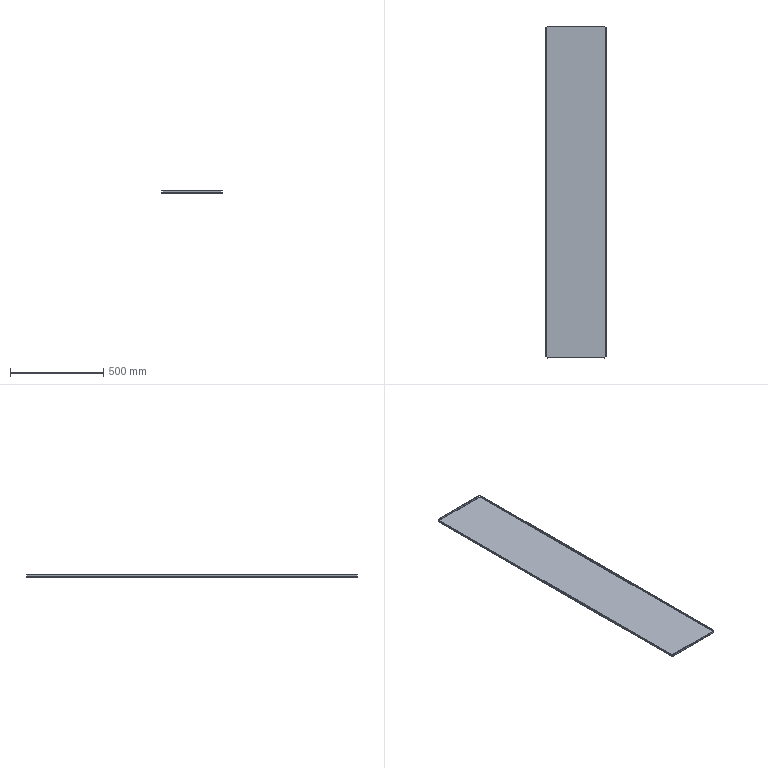Part | SolidWorks | features BaseBody 1 | 1 solid | 50 faces | box 322 x 1776 x 12 mm | volume 1518935 mm3 | plane 42 | cylinder 8 | commonest cylinder face diameters 1.473 x4 6.473 x4
STEP:
#1=CARTESIAN_POINT('',(-154.,885.5,9.5));
#2=VERTEX_POINT('',#1);
#3=CARTESIAN_POINT('',(154.,885.5,9.5));
#4=VERTEX_POINT('',#3);
#5=CARTESIAN_POINT('',(154.,885.5,9.5));
#6=DIRECTION('',(1.,0.,0.));
#7=VECTOR('',#6,1000.);
#8=LINE('',#5,#7);
#9=EDGE_CURVE('',#2,#4,#8,.T.);
#10=ORIENTED_EDGE('',*,*,#9,.T.);
#11=CARTESIAN_POINT('',(154.,888.,9.5));
#12=VERTEX_POINT('',#11);
#13=CARTESIAN_POINT('',(154.,888.,9.5));
#14=DIRECTION('',(0.,-1.,0.));
#15=VECTOR('',#14,1000.);
#16=LINE('',#13,#15);
#17=EDGE_CURVE('',#12,#4,#16,.T.);
#18=ORIENTED_EDGE('',*,*,#17,.F.);
#19=CARTESIAN_POINT('',(-154.,888.,9.5));
#20=VERTEX_POINT('',#19);
#21=CARTESIAN_POINT('',(0.,888.,9.5));
#22=DIRECTION('',(1.,0.,0.));
#23=VECTOR('',#22,1000.);
#24=LINE('',#21,#23);
#25=EDGE_CURVE('',#20,#12,#24,.T.);
#26=ORIENTED_EDGE('',*,*,#25,.F.);
#27=CARTESIAN_POINT('',(-154.,888.,9.5));
#28=DIRECTION('',(0.,-1.,0.));
#29=VECTOR('',#28,1000.);
#30=LINE('',#27,#29);
#31=EDGE_CURVE('',#20,#2,#30,.T.);
#32=ORIENTED_EDGE('',*,*,#31,.T.);
#33=EDGE_LOOP('',(#10,#18,#26,#32));
#34=FACE_OUTER_BOUND('',#33,.T.);
#35=CARTESIAN_POINT('',(154.,888.,9.5));
#36=DIRECTION('',(0.,0.,-1.));
#37=DIRECTION('',(0.,-1.,0.));
#38=AXIS2_PLACEMENT_3D('',#35,#36,#37);
#39=PLANE('',#38);
#40=ADVANCED_FACE('',(#34),#39,.F.);
#41=CARTESIAN_POINT('',(-154.,885.5,0.7366));
#42=VERTEX_POINT('',#41);
#43=CARTESIAN_POINT('',(-154.,885.5,9.5));
#44=DIRECTION('',(0.,0.,1.));
#45=VECTOR('',#44,1000.);
#46=LINE('',#43,#45);
#47=EDGE_CURVE('',#42,#2,#46,.T.);
#48=ORIENTED_EDGE('',*,*,#47,.F.);
#49=CARTESIAN_POINT('',(154.,885.5,0.7366));
#50=VERTEX_POINT('',#49);
#51=CARTESIAN_POINT('',(154.,885.5,0.7366));
#52=DIRECTION('',(-1.,0.,0.));
#53=VECTOR('',#52,1000.);
#54=LINE('',#51,#53);
#55=EDGE_CURVE('',#50,#42,#54,.T.);
#56=ORIENTED_EDGE('',*,*,#55,.F.);
#57=CARTESIAN_POINT('',(154.,885.5,0.));
#58=DIRECTION('',(0.,0.,-1.));
#59=VECTOR('',#58,1000.);
#60=LINE('',#57,#59);
#61=EDGE_CURVE('',#4,#50,#60,.T.);
#62=ORIENTED_EDGE('',*,*,#61,.F.);
#63=ORIENTED_EDGE('',*,*,#9,.F.);
#64=EDGE_LOOP('',(#48,#56,#62,#63));
#65=FACE_OUTER_BOUND('',#64,.T.);
#66=CARTESIAN_POINT('',(0.,885.5,0.));
#67=DIRECTION('',(0.,-1.,0.));
#68=DIRECTION('',(-1.,0.,0.));
#69=AXIS2_PLACEMENT_3D('',#66,#67,#68);
#70=PLANE('',#69);
#71=ADVANCED_FACE('',(#65),#70,.T.);
#72=CARTESIAN_POINT('',(-154.,888.,0.7366));
#73=VERTEX_POINT('',#72);
#74=CARTESIAN_POINT('',(154.,888.,0.7366));
#75=VERTEX_POINT('',#74);
#76=CARTESIAN_POINT('',(154.,888.,0.7366));
#77=DIRECTION('',(1.,0.,0.));
#78=VECTOR('',#77,1000.);
#79=LINE('',#76,#78);
#80=EDGE_CURVE('',#73,#75,#79,.T.);
#81=ORIENTED_EDGE('',*,*,#80,.F.);
#82=CARTESIAN_POINT('',(-154.,888.,0.));
#83=DIRECTION('',(0.,0.,1.));
#84=VECTOR('',#83,1000.);
#85=LINE('',#82,#84);
#86=EDGE_CURVE('',#73,#20,#85,.T.);
#87=ORIENTED_EDGE('',*,*,#86,.T.);
#88=ORIENTED_EDGE('',*,*,#25,.T.);
#89=CARTESIAN_POINT('',(154.,888.,0.));
#90=DIRECTION('',(0.,0.,-1.));
#91=VECTOR('',#90,1000.);
#92=LINE('',#89,#91);
#93=EDGE_CURVE('',#12,#75,#92,.T.);
#94=ORIENTED_EDGE('',*,*,#93,.T.);
#95=EDGE_LOOP('',(#81,#87,#88,#94));
#96=FACE_OUTER_BOUND('',#95,.T.);
#97=CARTESIAN_POINT('',(0.,888.,0.));
#98=DIRECTION('',(0.,-1.,0.));
#99=DIRECTION('',(-1.,0.,0.));
#100=AXIS2_PLACEMENT_3D('',#97,#98,#99);
#101=PLANE('',#100);
#102=ADVANCED_FACE('',(#96),#101,.F.);
#103=CARTESIAN_POINT('',(-154.,885.5,0.7366));
#104=DIRECTION('',(0.,1.,0.));
#105=VECTOR('',#104,1000.);
#106=LINE('',#103,#105);
#107=EDGE_CURVE('',#42,#73,#106,.T.);
#108=ORIENTED_EDGE('',*,*,#107,.F.);
#109=ORIENTED_EDGE('',*,*,#47,.T.);
#110=ORIENTED_EDGE('',*,*,#31,.F.);
#111=ORIENTED_EDGE('',*,*,#86,.F.);
#112=EDGE_LOOP('',(#108,#109,#110,#111));
#113=FACE_OUTER_BOUND('',#112,.T.);
#114=CARTESIAN_POINT('',(-154.,888.,9.5));
#115=DIRECTION('',(1.,0.,0.));
#116=DIRECTION('',(0.,0.,-1.));
#117=AXIS2_PLACEMENT_3D('',#114,#115,#116);
#118=PLANE('',#117);
#119=ADVANCED_FACE('',(#113),#118,.F.);
#120=CARTESIAN_POINT('',(154.,888.,0.7366));
#121=DIRECTION('',(0.,1.,0.));
#122=VECTOR('',#121,1000.);
#123=LINE('',#120,#122);
#124=EDGE_CURVE('',#50,#75,#123,.T.);
#125=ORIENTED_EDGE('',*,*,#124,.T.);
#126=ORIENTED_EDGE('',*,*,#93,.F.);
#127=ORIENTED_EDGE('',*,*,#17,.T.);
#128=ORIENTED_EDGE('',*,*,#61,.T.);
#129=EDGE_LOOP('',(#125,#126,#127,#128));
#130=FACE_OUTER_BOUND('',#129,.T.);
#131=CARTESIAN_POINT('',(154.,888.,0.));
#132=DIRECTION('',(-1.,0.,0.));
#133=DIRECTION('',(0.,0.,1.));
#134=AXIS2_PLACEMENT_3D('',#131,#132,#133);
#135=PLANE('',#134);
#136=ADVANCED_FACE('',(#130),#135,.F.);
#137=CARTESIAN_POINT('',(-154.,884.763,0.));
#138=VERTEX_POINT('',#137);
#139=CARTESIAN_POINT('',(154.,884.763,0.));
#140=VERTEX_POINT('',#139);
#141=CARTESIAN_POINT('',(-154.,884.763,0.));
#142=DIRECTION('',(1.,0.,0.));
#143=VECTOR('',#142,1000.);
#144=LINE('',#141,#143);
#145=EDGE_CURVE('',#138,#140,#144,.T.);
#146=ORIENTED_EDGE('',*,*,#145,.T.);
#147=CARTESIAN_POINT('',(154.,884.763,0.7366));
#148=DIRECTION('',(1.,0.,0.));
#149=DIRECTION('',(0.,0.,1.));
#150=AXIS2_PLACEMENT_3D('',#147,#148,#149);
#151=CIRCLE('',#150,0.7366);
#152=EDGE_CURVE('',#140,#50,#151,.T.);
#153=ORIENTED_EDGE('',*,*,#152,.T.);
#154=ORIENTED_EDGE('',*,*,#55,.T.);
#155=CARTESIAN_POINT('',(-154.,884.763,0.7366));
#156=DIRECTION('',(-1.,0.,0.));
#157=DIRECTION('',(0.,0.,1.));
#158=AXIS2_PLACEMENT_3D('',#155,#156,#157);
#159=CIRCLE('',#158,0.7366);
#160=EDGE_CURVE('',#42,#138,#159,.T.);
#161=ORIENTED_EDGE('',*,*,#160,.T.);
#162=EDGE_LOOP('',(#146,#153,#154,#161));
#163=FACE_OUTER_BOUND('',#162,.T.);
#164=CARTESIAN_POINT('',(-154.,884.763,0.7366));
#165=DIRECTION('',(-1.,0.,0.));
#166=DIRECTION('',(0.,1.,0.));
#167=AXIS2_PLACEMENT_3D('',#164,#165,#166);
#168=CYLINDRICAL_SURFACE('',#167,0.7366);
#169=ADVANCED_FACE('',(#163),#168,.F.);
#170=CARTESIAN_POINT('',(-154.,884.763,-2.5));
#171=VERTEX_POINT('',#170);
#172=CARTESIAN_POINT('',(154.,884.763,-2.5));
#173=VERTEX_POINT('',#172);
#174=CARTESIAN_POINT('',(-154.,884.763,-2.5));
#175=DIRECTION('',(1.,0.,0.));
#176=VECTOR('',#175,1000.);
#177=LINE('',#174,#176);
#178=EDGE_CURVE('',#171,#173,#177,.T.);
#179=ORIENTED_EDGE('',*,*,#178,.F.);
#180=CARTESIAN_POINT('',(-154.,887.915,0.));
#181=VERTEX_POINT('',#180);
#182=CARTESIAN_POINT('',(-154.,884.763,0.7366));
#183=DIRECTION('',(-1.,0.,0.));
#184=DIRECTION('',(0.,0.,1.));
#185=AXIS2_PLACEMENT_3D('',#182,#183,#184);
#186=CIRCLE('',#185,3.237);
#187=EDGE_CURVE('',#181,#171,#186,.T.);
#188=ORIENTED_EDGE('',*,*,#187,.F.);
#189=CARTESIAN_POINT('',(-154.,884.763,0.7366));
#190=DIRECTION('',(-1.,0.,0.));
#191=DIRECTION('',(0.,0.,1.));
#192=AXIS2_PLACEMENT_3D('',#189,#190,#191);
#193=CIRCLE('',#192,3.237);
#194=EDGE_CURVE('',#73,#181,#193,.T.);
#195=ORIENTED_EDGE('',*,*,#194,.F.);
#196=ORIENTED_EDGE('',*,*,#80,.T.);
#197=CARTESIAN_POINT('',(154.,887.915,0.));
#198=VERTEX_POINT('',#197);
#199=CARTESIAN_POINT('',(154.,884.763,0.7366));
#200=DIRECTION('',(1.,0.,0.));
#201=DIRECTION('',(0.,0.,1.));
#202=AXIS2_PLACEMENT_3D('',#199,#200,#201);
#203=CIRCLE('',#202,3.237);
#204=EDGE_CURVE('',#198,#75,#203,.T.);
#205=ORIENTED_EDGE('',*,*,#204,.F.);
#206=CARTESIAN_POINT('',(154.,884.763,0.7366));
#207=DIRECTION('',(1.,0.,0.));
#208=DIRECTION('',(0.,0.,1.));
#209=AXIS2_PLACEMENT_3D('',#206,#207,#208);
#210=CIRCLE('',#209,3.237);
#211=EDGE_CURVE('',#173,#198,#210,.T.);
#212=ORIENTED_EDGE('',*,*,#211,.F.);
#213=EDGE_LOOP('',(#179,#188,#195,#196,#205,#212));
#214=FACE_OUTER_BOUND('',#213,.T.);
#215=CARTESIAN_POINT('',(-154.,884.763,0.7366));
#216=DIRECTION('',(-1.,0.,0.));
#217=DIRECTION('',(0.,1.,0.));
#218=AXIS2_PLACEMENT_3D('',#215,#216,#217);
#219=CYLINDRICAL_SURFACE('',#218,3.237);
#220=ADVANCED_FACE('',(#214),#219,.T.);
#221=ORIENTED_EDGE('',*,*,#194,.T.);
#222=CARTESIAN_POINT('',(-154.,888.,0.));
#223=DIRECTION('',(0.,-1.,0.));
#224=VECTOR('',#223,1000.);
#225=LINE('',#222,#224);
#226=EDGE_CURVE('',#181,#138,#225,.T.);
#227=ORIENTED_EDGE('',*,*,#226,.T.);
#228=ORIENTED_EDGE('',*,*,#160,.F.);
#229=ORIENTED_EDGE('',*,*,#107,.T.);
#230=EDGE_LOOP('',(#221,#227,#228,#229));
#231=FACE_OUTER_BOUND('',#230,.T.);
#232=CARTESIAN_POINT('',(-154.,884.763,0.7366));
#233=DIRECTION('',(1.,0.,0.));
#234=DIRECTION('',(0.,0.,-1.));
#235=AXIS2_PLACEMENT_3D('',#232,#233,#234);
#236=PLANE('',#235);
#237=ADVANCED_FACE('',(#231),#236,.F.);
#238=ORIENTED_EDGE('',*,*,#152,.F.);
#239=CARTESIAN_POINT('',(154.,884.763,0.));
#240=DIRECTION('',(0.,1.,0.));
#241=VECTOR('',#240,1000.);
#242=LINE('',#239,#241);
#243=EDGE_CURVE('',#140,#198,#242,.T.);
#244=ORIENTED_EDGE('',*,*,#243,.T.);
#245=ORIENTED_EDGE('',*,*,#204,.T.);
#246=ORIENTED_EDGE('',*,*,#124,.F.);
#247=EDGE_LOOP('',(#238,#244,#245,#246));
#248=FACE_OUTER_BOUND('',#247,.T.);
#249=CARTESIAN_POINT('',(154.,884.763,0.7366));
#250=DIRECTION('',(1.,0.,0.));
#251=DIRECTION('',(0.,0.,-1.));
#252=AXIS2_PLACEMENT_3D('',#249,#250,#251);
#253=PLANE('',#252);
#254=ADVANCED_FACE('',(#248),#253,.T.);
#255=CARTESIAN_POINT('',(158.5,881.,9.5));
#256=VERTEX_POINT('',#255);
#257=CARTESIAN_POINT('',(158.5,-881.,9.5));
#258=VERTEX_POINT('',#257);
#259=CARTESIAN_POINT('',(158.5,-881.,9.5));
#260=DIRECTION('',(0.,-1.,0.));
#261=VECTOR('',#260,1000.);
#262=LINE('',#259,#261);
#263=EDGE_CURVE('',#256,#258,#262,.T.);
#264=ORIENTED_EDGE('',*,*,#263,.T.);
#265=CARTESIAN_POINT('',(161.,-881.,9.5));
#266=VERTEX_POINT('',#265);
#267=CARTESIAN_POINT('',(161.,-881.,9.5));
#268=DIRECTION('',(-1.,0.,0.));
#269=VECTOR('',#268,1000.);
#270=LINE('',#267,#269);
#271=EDGE_CURVE('',#266,#258,#270,.T.);
#272=ORIENTED_EDGE('',*,*,#271,.F.);
#273=CARTESIAN_POINT('',(161.,881.,9.5));
#274=VERTEX_POINT('',#273);
#275=CARTESIAN_POINT('',(161.,0.,9.5));
#276=DIRECTION('',(0.,-1.,0.));
#277=VECTOR('',#276,1000.);
#278=LINE('',#275,#277);
#279=EDGE_CURVE('',#274,#266,#278,.T.);
#280=ORIENTED_EDGE('',*,*,#279,.F.);
#281=CARTESIAN_POINT('',(161.,881.,9.5));
#282=DIRECTION('',(-1.,0.,0.));
#283=VECTOR('',#282,1000.);
#284=LINE('',#281,#283);
#285=EDGE_CURVE('',#274,#256,#284,.T.);
#286=ORIENTED_EDGE('',*,*,#285,.T.);
#287=EDGE_LOOP('',(#264,#272,#280,#286));
#288=FACE_OUTER_BOUND('',#287,.T.);
#289=CARTESIAN_POINT('',(161.,-881.,9.5));
#290=DIRECTION('',(0.,0.,-1.));
#291=DIRECTION('',(-1.,0.,0.));
#292=AXIS2_PLACEMENT_3D('',#289,#290,#291);
#293=PLANE('',#292);
#294=ADVANCED_FACE('',(#288),#293,.F.);
#295=CARTESIAN_POINT('',(158.5,881.,0.7366));
#296=VERTEX_POINT('',#295);
#297=CARTESIAN_POINT('',(158.5,881.,9.5));
#298=DIRECTION('',(0.,0.,1.));
#299=VECTOR('',#298,1000.);
#300=LINE('',#297,#299);
#301=EDGE_CURVE('',#296,#256,#300,.T.);
#302=ORIENTED_EDGE('',*,*,#301,.F.);
#303=CARTESIAN_POINT('',(158.5,-881.,0.7366));
#304=VERTEX_POINT('',#303);
#305=CARTESIAN_POINT('',(158.5,-881.,0.7366));
#306=DIRECTION('',(0.,1.,0.));
#307=VECTOR('',#306,1000.);
#308=LINE('',#305,#307);
#309=EDGE_CURVE('',#304,#296,#308,.T.);
#310=ORIENTED_EDGE('',*,*,#309,.F.);
#311=CARTESIAN_POINT('',(158.5,-881.,0.));
#312=DIRECTION('',(0.,0.,-1.));
#313=VECTOR('',#312,1000.);
#314=LINE('',#311,#313);
#315=EDGE_CURVE('',#258,#304,#314,.T.);
#316=ORIENTED_EDGE('',*,*,#315,.F.);
#317=ORIENTED_EDGE('',*,*,#263,.F.);
#318=EDGE_LOOP('',(#302,#310,#316,#317));
#319=FACE_OUTER_BOUND('',#318,.T.);
#320=CARTESIAN_POINT('',(158.5,0.,0.));
#321=DIRECTION('',(-1.,0.,0.));
#322=DIRECTION('',(0.,1.,0.));
#323=AXIS2_PLACEMENT_3D('',#320,#321,#322);
#324=PLANE('',#323);
#325=ADVANCED_FACE('',(#319),#324,.T.);
#326=CARTESIAN_POINT('',(161.,881.,0.7366));
#327=VERTEX_POINT('',#326);
#328=CARTESIAN_POINT('',(161.,-881.,0.7366));
#329=VERTEX_POINT('',#328);
#330=CARTESIAN_POINT('',(161.,-881.,0.7366));
#331=DIRECTION('',(0.,-1.,0.));
#332=VECTOR('',#331,1000.);
#333=LINE('',#330,#332);
#334=EDGE_CURVE('',#327,#329,#333,.T.);
#335=ORIENTED_EDGE('',*,*,#334,.F.);
#336=CARTESIAN_POINT('',(161.,881.,0.));
#337=DIRECTION('',(0.,0.,1.));
#338=VECTOR('',#337,1000.);
#339=LINE('',#336,#338);
#340=EDGE_CURVE('',#327,#274,#339,.T.);
#341=ORIENTED_EDGE('',*,*,#340,.T.);
#342=ORIENTED_EDGE('',*,*,#279,.T.);
#343=CARTESIAN_POINT('',(161.,-881.,0.));
#344=DIRECTION('',(0.,0.,-1.));
#345=VECTOR('',#344,1000.);
#346=LINE('',#343,#345);
#347=EDGE_CURVE('',#266,#329,#346,.T.);
#348=ORIENTED_EDGE('',*,*,#347,.T.);
#349=EDGE_LOOP('',(#335,#341,#342,#348));
#350=FACE_OUTER_BOUND('',#349,.T.);
#351=CARTESIAN_POINT('',(161.,0.,0.));
#352=DIRECTION('',(-1.,0.,0.));
#353=DIRECTION('',(0.,1.,0.));
#354=AXIS2_PLACEMENT_3D('',#351,#352,#353);
#355=PLANE('',#354);
#356=ADVANCED_FACE('',(#350),#355,.F.);
#357=CARTESIAN_POINT('',(158.5,881.,0.7366));
#358=DIRECTION('',(1.,0.,0.));
#359=VECTOR('',#358,1000.);
#360=LINE('',#357,#359);
#361=EDGE_CURVE('',#296,#327,#360,.T.);
#362=ORIENTED_EDGE('',*,*,#361,.F.);
#363=ORIENTED_EDGE('',*,*,#301,.T.);
#364=ORIENTED_EDGE('',*,*,#285,.F.);
#365=ORIENTED_EDGE('',*,*,#340,.F.);
#366=EDGE_LOOP('',(#362,#363,#364,#365));
#367=FACE_OUTER_BOUND('',#366,.T.);
#368=CARTESIAN_POINT('',(161.,881.,9.5));
#369=DIRECTION('',(0.,-1.,0.));
#370=DIRECTION('',(0.,0.,-1.));
#371=AXIS2_PLACEMENT_3D('',#368,#369,#370);
#372=PLANE('',#371);
#373=ADVANCED_FACE('',(#367),#372,.F.);
#374=CARTESIAN_POINT('',(161.,-881.,0.7366));
#375=DIRECTION('',(1.,0.,0.));
#376=VECTOR('',#375,1000.);
#377=LINE('',#374,#376);
#378=EDGE_CURVE('',#304,#329,#377,.T.);
#379=ORIENTED_EDGE('',*,*,#378,.T.);
#380=ORIENTED_EDGE('',*,*,#347,.F.);
#381=ORIENTED_EDGE('',*,*,#271,.T.);
#382=ORIENTED_EDGE('',*,*,#315,.T.);
#383=EDGE_LOOP('',(#379,#380,#381,#382));
#384=FACE_OUTER_BOUND('',#383,.T.);
#385=CARTESIAN_POINT('',(161.,-881.,0.));
#386=DIRECTION('',(0.,1.,0.));
#387=DIRECTION('',(1.,0.,0.));
#388=AXIS2_PLACEMENT_3D('',#385,#386,#387);
#389=PLANE('',#388);
#390=ADVANCED_FACE('',(#384),#389,.F.);
#391=CARTESIAN_POINT('',(157.763,881.,0.));
#392=VERTEX_POINT('',#391);
#393=CARTESIAN_POINT('',(157.763,-881.,0.));
#394=VERTEX_POINT('',#393);
#395=CARTESIAN_POINT('',(157.763,881.,0.));
#396=DIRECTION('',(0.,-1.,0.));
#397=VECTOR('',#396,1000.);
#398=LINE('',#395,#397);
#399=EDGE_CURVE('',#392,#394,#398,.T.);
#400=ORIENTED_EDGE('',*,*,#399,.T.);
#401=CARTESIAN_POINT('',(157.763,-881.,0.7366));
#402=DIRECTION('',(0.,-1.,0.));
#403=DIRECTION('',(0.,0.,1.));
#404=AXIS2_PLACEMENT_3D('',#401,#402,#403);
#405=CIRCLE('',#404,0.7366);
#406=EDGE_CURVE('',#394,#304,#405,.T.);
#407=ORIENTED_EDGE('',*,*,#406,.T.);
#408=ORIENTED_EDGE('',*,*,#309,.T.);
#409=CARTESIAN_POINT('',(157.763,881.,0.7366));
#410=DIRECTION('',(0.,1.,0.));
#411=DIRECTION('',(0.,0.,1.));
#412=AXIS2_PLACEMENT_3D('',#409,#410,#411);
#413=CIRCLE('',#412,0.7366);
#414=EDGE_CURVE('',#296,#392,#413,.T.);
#415=ORIENTED_EDGE('',*,*,#414,.T.);
#416=EDGE_LOOP('',(#400,#407,#408,#415));
#417=FACE_OUTER_BOUND('',#416,.T.);
#418=CARTESIAN_POINT('',(157.763,881.,0.7366));
#419=DIRECTION('',(0.,1.,0.));
#420=DIRECTION('',(1.,0.,0.));
#421=AXIS2_PLACEMENT_3D('',#418,#419,#420);
#422=CYLINDRICAL_SURFACE('',#421,0.7366);
#423=ADVANCED_FACE('',(#417),#422,.F.);
#424=CARTESIAN_POINT('',(157.763,881.,-2.5));
#425=VERTEX_POINT('',#424);
#426=CARTESIAN_POINT('',(157.763,-881.,-2.5));
#427=VERTEX_POINT('',#426);
#428=CARTESIAN_POINT('',(157.763,881.,-2.5));
#429=DIRECTION('',(0.,-1.,0.));
#430=VECTOR('',#429,1000.);
#431=LINE('',#428,#430);
#432=EDGE_CURVE('',#425,#427,#431,.T.);
#433=ORIENTED_EDGE('',*,*,#432,.F.);
#434=CARTESIAN_POINT('',(160.915,881.,0.));
#435=VERTEX_POINT('',#434);
#436=CARTESIAN_POINT('',(157.763,881.,0.7366));
#437=DIRECTION('',(0.,1.,0.));
#438=DIRECTION('',(0.,0.,1.));
#439=AXIS2_PLACEMENT_3D('',#436,#437,#438);
#440=CIRCLE('',#439,3.237);
#441=EDGE_CURVE('',#435,#425,#440,.T.);
#442=ORIENTED_EDGE('',*,*,#441,.F.);
#443=CARTESIAN_POINT('',(157.763,881.,0.7366));
#444=DIRECTION('',(0.,1.,0.));
#445=DIRECTION('',(0.,0.,1.));
#446=AXIS2_PLACEMENT_3D('',#443,#444,#445);
#447=CIRCLE('',#446,3.237);
#448=EDGE_CURVE('',#327,#435,#447,.T.);
#449=ORIENTED_EDGE('',*,*,#448,.F.);
#450=ORIENTED_EDGE('',*,*,#334,.T.);
#451=CARTESIAN_POINT('',(160.915,-881.,0.));
#452=VERTEX_POINT('',#451);
#453=CARTESIAN_POINT('',(157.763,-881.,0.7366));
#454=DIRECTION('',(0.,-1.,0.));
#455=DIRECTION('',(0.,0.,1.));
#456=AXIS2_PLACEMENT_3D('',#453,#454,#455);
#457=CIRCLE('',#456,3.237);
#458=EDGE_CURVE('',#452,#329,#457,.T.);
#459=ORIENTED_EDGE('',*,*,#458,.F.);
#460=CARTESIAN_POINT('',(157.763,-881.,0.7366));
#461=DIRECTION('',(0.,-1.,0.));
#462=DIRECTION('',(0.,0.,1.));
#463=AXIS2_PLACEMENT_3D('',#460,#461,#462);
#464=CIRCLE('',#463,3.237);
#465=EDGE_CURVE('',#427,#452,#464,.T.);
#466=ORIENTED_EDGE('',*,*,#465,.F.);
#467=EDGE_LOOP('',(#433,#442,#449,#450,#459,#466));
#468=FACE_OUTER_BOUND('',#467,.T.);
#469=CARTESIAN_POINT('',(157.763,881.,0.7366));
#470=DIRECTION('',(0.,1.,0.));
#471=DIRECTION('',(1.,0.,0.));
#472=AXIS2_PLACEMENT_3D('',#469,#470,#471);
#473=CYLINDRICAL_SURFACE('',#472,3.237);
#474=ADVANCED_FACE('',(#468),#473,.T.);
#475=ORIENTED_EDGE('',*,*,#448,.T.);
#476=CARTESIAN_POINT('',(161.,881.,0.));
#477=DIRECTION('',(-1.,0.,0.));
#478=VECTOR('',#477,1000.);
#479=LINE('',#476,#478);
#480=EDGE_CURVE('',#435,#392,#479,.T.);
#481=ORIENTED_EDGE('',*,*,#480,.T.);
#482=ORIENTED_EDGE('',*,*,#414,.F.);
#483=ORIENTED_EDGE('',*,*,#361,.T.);
#484=EDGE_LOOP('',(#475,#481,#482,#483));
#485=FACE_OUTER_BOUND('',#484,.T.);
#486=CARTESIAN_POINT('',(157.763,881.,0.7366));
#487=DIRECTION('',(0.,-1.,0.));
#488=DIRECTION('',(0.,0.,-1.));
#489=AXIS2_PLACEMENT_3D('',#486,#487,#488);
#490=PLANE('',#489);
#491=ADVANCED_FACE('',(#485),#490,.F.);
#492=ORIENTED_EDGE('',*,*,#406,.F.);
#493=CARTESIAN_POINT('',(157.763,-881.,0.));
#494=DIRECTION('',(1.,0.,0.));
#495=VECTOR('',#494,1000.);
#496=LINE('',#493,#495);
#497=EDGE_CURVE('',#394,#452,#496,.T.);
#498=ORIENTED_EDGE('',*,*,#497,.T.);
#499=ORIENTED_EDGE('',*,*,#458,.T.);
#500=ORIENTED_EDGE('',*,*,#378,.F.);
#501=EDGE_LOOP('',(#492,#498,#499,#500));
#502=FACE_OUTER_BOUND('',#501,.T.);
#503=CARTESIAN_POINT('',(157.763,-881.,0.7366));
#504=DIRECTION('',(0.,-1.,0.));
#505=DIRECTION('',(0.,0.,-1.));
#506=AXIS2_PLACEMENT_3D('',#503,#504,#505);
#507=PLANE('',#506);
#508=ADVANCED_FACE('',(#502),#507,.T.);
#509=CARTESIAN_POINT('',(154.,-885.5,9.5));
#510=VERTEX_POINT('',#509);
#511=CARTESIAN_POINT('',(-154.,-885.5,9.5));
#512=VERTEX_POINT('',#511);
#513=CARTESIAN_POINT('',(-154.,-885.5,9.5));
#514=DIRECTION('',(-1.,0.,0.));
#515=VECTOR('',#514,1000.);
#516=LINE('',#513,#515);
#517=EDGE_CURVE('',#510,#512,#516,.T.);
#518=ORIENTED_EDGE('',*,*,#517,.T.);
#519=CARTESIAN_POINT('',(-154.,-888.,9.5));
#520=VERTEX_POINT('',#519);
#521=CARTESIAN_POINT('',(-154.,-888.,9.5));
#522=DIRECTION('',(0.,1.,0.));
#523=VECTOR('',#522,1000.);
#524=LINE('',#521,#523);
#525=EDGE_CURVE('',#520,#512,#524,.T.);
#526=ORIENTED_EDGE('',*,*,#525,.F.);
#527=CARTESIAN_POINT('',(154.,-888.,9.5));
#528=VERTEX_POINT('',#527);
#529=CARTESIAN_POINT('',(0.,-888.,9.5));
#530=DIRECTION('',(-1.,0.,0.));
#531=VECTOR('',#530,1000.);
#532=LINE('',#529,#531);
#533=EDGE_CURVE('',#528,#520,#532,.T.);
#534=ORIENTED_EDGE('',*,*,#533,.F.);
#535=CARTESIAN_POINT('',(154.,-888.,9.5));
#536=DIRECTION('',(0.,1.,0.));
#537=VECTOR('',#536,1000.);
#538=LINE('',#535,#537);
#539=EDGE_CURVE('',#528,#510,#538,.T.);
#540=ORIENTED_EDGE('',*,*,#539,.T.);
#541=EDGE_LOOP('',(#518,#526,#534,#540));
#542=FACE_OUTER_BOUND('',#541,.T.);
#543=CARTESIAN_POINT('',(-154.,-888.,9.5));
#544=DIRECTION('',(0.,0.,-1.));
#545=DIRECTION('',(-1.,0.,0.));
#546=AXIS2_PLACEMENT_3D('',#543,#544,#545);
#547=PLANE('',#546);
#548=ADVANCED_FACE('',(#542),#547,.F.);
#549=CARTESIAN_POINT('',(154.,-885.5,0.7366));
#550=VERTEX_POINT('',#549);
#551=CARTESIAN_POINT('',(154.,-885.5,9.5));
#552=DIRECTION('',(0.,0.,1.));
#553=VECTOR('',#552,1000.);
#554=LINE('',#551,#553);
#555=EDGE_CURVE('',#550,#510,#554,.T.);
#556=ORIENTED_EDGE('',*,*,#555,.F.);
#557=CARTESIAN_POINT('',(-154.,-885.5,0.7366));
#558=VERTEX_POINT('',#557);
#559=CARTESIAN_POINT('',(-154.,-885.5,0.7366));
#560=DIRECTION('',(1.,0.,0.));
#561=VECTOR('',#560,1000.);
#562=LINE('',#559,#561);
#563=EDGE_CURVE('',#558,#550,#562,.T.);
#564=ORIENTED_EDGE('',*,*,#563,.F.);
#565=CARTESIAN_POINT('',(-154.,-885.5,0.));
#566=DIRECTION('',(0.,0.,-1.));
#567=VECTOR('',#566,1000.);
#568=LINE('',#565,#567);
#569=EDGE_CURVE('',#512,#558,#568,.T.);
#570=ORIENTED_EDGE('',*,*,#569,.F.);
#571=ORIENTED_EDGE('',*,*,#517,.F.);
#572=EDGE_LOOP('',(#556,#564,#570,#571));
#573=FACE_OUTER_BOUND('',#572,.T.);
#574=CARTESIAN_POINT('',(0.,-885.5,0.));
#575=DIRECTION('',(0.,1.,0.));
#576=DIRECTION('',(0.,0.,-1.));
#577=AXIS2_PLACEMENT_3D('',#574,#575,#576);
#578=PLANE('',#577);
#579=ADVANCED_FACE('',(#573),#578,.T.);
#580=CARTESIAN_POINT('',(154.,-888.,0.7366));
#581=VERTEX_POINT('',#580);
#582=CARTESIAN_POINT('',(-154.,-888.,0.7366));
#583=VERTEX_POINT('',#582);
#584=CARTESIAN_POINT('',(-154.,-888.,0.7366));
#585=DIRECTION('',(-1.,0.,0.));
#586=VECTOR('',#585,1000.);
#587=LINE('',#584,#586);
#588=EDGE_CURVE('',#581,#583,#587,.T.);
#589=ORIENTED_EDGE('',*,*,#588,.F.);
#590=CARTESIAN_POINT('',(154.,-888.,0.));
#591=DIRECTION('',(0.,0.,1.));
#592=VECTOR('',#591,1000.);
#593=LINE('',#590,#592);
#594=EDGE_CURVE('',#581,#528,#593,.T.);
#595=ORIENTED_EDGE('',*,*,#594,.T.);
#596=ORIENTED_EDGE('',*,*,#533,.T.);
#597=CARTESIAN_POINT('',(-154.,-888.,0.));
#598=DIRECTION('',(0.,0.,-1.));
#599=VECTOR('',#598,1000.);
#600=LINE('',#597,#599);
#601=EDGE_CURVE('',#520,#583,#600,.T.);
#602=ORIENTED_EDGE('',*,*,#601,.T.);
#603=EDGE_LOOP('',(#589,#595,#596,#602));
#604=FACE_OUTER_BOUND('',#603,.T.);
#605=CARTESIAN_POINT('',(0.,-888.,0.));
#606=DIRECTION('',(0.,1.,0.));
#607=DIRECTION('',(0.,0.,-1.));
#608=AXIS2_PLACEMENT_3D('',#605,#606,#607);
#609=PLANE('',#608);
#610=ADVANCED_FACE('',(#604),#609,.F.);
#611=CARTESIAN_POINT('',(154.,-885.5,0.7366));
#612=DIRECTION('',(0.,-1.,0.));
#613=VECTOR('',#612,1000.);
#614=LINE('',#611,#613);
#615=EDGE_CURVE('',#550,#581,#614,.T.);
#616=ORIENTED_EDGE('',*,*,#615,.F.);
#617=ORIENTED_EDGE('',*,*,#555,.T.);
#618=ORIENTED_EDGE('',*,*,#539,.F.);
#619=ORIENTED_EDGE('',*,*,#594,.F.);
#620=EDGE_LOOP('',(#616,#617,#618,#619));
#621=FACE_OUTER_BOUND('',#620,.T.);
#622=CARTESIAN_POINT('',(154.,-888.,9.5));
#623=DIRECTION('',(-1.,0.,0.));
#624=DIRECTION('',(0.,1.,0.));
#625=AXIS2_PLACEMENT_3D('',#622,#623,#624);
#626=PLANE('',#625);
#627=ADVANCED_FACE('',(#621),#626,.F.);
#628=CARTESIAN_POINT('',(-154.,-888.,0.7366));
#629=DIRECTION('',(0.,-1.,0.));
#630=VECTOR('',#629,1000.);
#631=LINE('',#628,#630);
#632=EDGE_CURVE('',#558,#583,#631,.T.);
#633=ORIENTED_EDGE('',*,*,#632,.T.);
#634=ORIENTED_EDGE('',*,*,#601,.F.);
#635=ORIENTED_EDGE('',*,*,#525,.T.);
#636=ORIENTED_EDGE('',*,*,#569,.T.);
#637=EDGE_LOOP('',(#633,#634,#635,#636));
#638=FACE_OUTER_BOUND('',#637,.T.);
#639=CARTESIAN_POINT('',(-154.,-888.,0.));
#640=DIRECTION('',(1.,0.,0.));
#641=DIRECTION('',(0.,0.,-1.));
#642=AXIS2_PLACEMENT_3D('',#639,#640,#641);
#643=PLANE('',#642);
#644=ADVANCED_FACE('',(#638),#643,.F.);
#645=CARTESIAN_POINT('',(154.,-884.763,0.));
#646=VERTEX_POINT('',#645);
#647=CARTESIAN_POINT('',(-154.,-884.763,0.));
#648=VERTEX_POINT('',#647);
#649=CARTESIAN_POINT('',(154.,-884.763,0.));
#650=DIRECTION('',(-1.,0.,0.));
#651=VECTOR('',#650,1000.);
#652=LINE('',#649,#651);
#653=EDGE_CURVE('',#646,#648,#652,.T.);
#654=ORIENTED_EDGE('',*,*,#653,.T.);
#655=CARTESIAN_POINT('',(-154.,-884.763,0.7366));
#656=DIRECTION('',(-1.,0.,0.));
#657=DIRECTION('',(0.,0.,-1.));
#658=AXIS2_PLACEMENT_3D('',#655,#656,#657);
#659=CIRCLE('',#658,0.7366);
#660=EDGE_CURVE('',#648,#558,#659,.T.);
#661=ORIENTED_EDGE('',*,*,#660,.T.);
#662=ORIENTED_EDGE('',*,*,#563,.T.);
#663=CARTESIAN_POINT('',(154.,-884.763,0.7366));
#664=DIRECTION('',(1.,0.,0.));
#665=DIRECTION('',(0.,0.,-1.));
#666=AXIS2_PLACEMENT_3D('',#663,#664,#665);
#667=CIRCLE('',#666,0.7366);
#668=EDGE_CURVE('',#550,#646,#667,.T.);
#669=ORIENTED_EDGE('',*,*,#668,.T.);
#670=EDGE_LOOP('',(#654,#661,#662,#669));
#671=FACE_OUTER_BOUND('',#670,.T.);
#672=CARTESIAN_POINT('',(154.,-884.763,0.7366));
#673=DIRECTION('',(1.,0.,0.));
#674=DIRECTION('',(0.,-1.,0.));
#675=AXIS2_PLACEMENT_3D('',#672,#673,#674);
#676=CYLINDRICAL_SURFACE('',#675,0.7366);
#677=ADVANCED_FACE('',(#671),#676,.F.);
#678=CARTESIAN_POINT('',(154.,-884.763,-2.5));
#679=VERTEX_POINT('',#678);
#680=CARTESIAN_POINT('',(-154.,-884.763,-2.5));
#681=VERTEX_POINT('',#680);
#682=CARTESIAN_POINT('',(154.,-884.763,-2.5));
#683=DIRECTION('',(-1.,0.,0.));
#684=VECTOR('',#683,1000.);
#685=LINE('',#682,#684);
#686=EDGE_CURVE('',#679,#681,#685,.T.);
#687=ORIENTED_EDGE('',*,*,#686,.F.);
#688=CARTESIAN_POINT('',(154.,-887.915,0.));
#689=VERTEX_POINT('',#688);
#690=CARTESIAN_POINT('',(154.,-884.763,0.7366));
#691=DIRECTION('',(1.,0.,0.));
#692=DIRECTION('',(0.,0.,-1.));
#693=AXIS2_PLACEMENT_3D('',#690,#691,#692);
#694=CIRCLE('',#693,3.237);
#695=EDGE_CURVE('',#689,#679,#694,.T.);
#696=ORIENTED_EDGE('',*,*,#695,.F.);
#697=CARTESIAN_POINT('',(154.,-884.763,0.7366));
#698=DIRECTION('',(1.,0.,0.));
#699=DIRECTION('',(0.,0.,-1.));
#700=AXIS2_PLACEMENT_3D('',#697,#698,#699);
#701=CIRCLE('',#700,3.237);
#702=EDGE_CURVE('',#581,#689,#701,.T.);
#703=ORIENTED_EDGE('',*,*,#702,.F.);
#704=ORIENTED_EDGE('',*,*,#588,.T.);
#705=CARTESIAN_POINT('',(-154.,-887.915,0.));
#706=VERTEX_POINT('',#705);
#707=CARTESIAN_POINT('',(-154.,-884.763,0.7366));
#708=DIRECTION('',(-1.,0.,0.));
#709=DIRECTION('',(0.,0.,-1.));
#710=AXIS2_PLACEMENT_3D('',#707,#708,#709);
#711=CIRCLE('',#710,3.237);
#712=EDGE_CURVE('',#706,#583,#711,.T.);
#713=ORIENTED_EDGE('',*,*,#712,.F.);
#714=CARTESIAN_POINT('',(-154.,-884.763,0.7366));
#715=DIRECTION('',(-1.,0.,0.));
#716=DIRECTION('',(0.,0.,-1.));
#717=AXIS2_PLACEMENT_3D('',#714,#715,#716);
#718=CIRCLE('',#717,3.237);
#719=EDGE_CURVE('',#681,#706,#718,.T.);
#720=ORIENTED_EDGE('',*,*,#719,.F.);
#721=EDGE_LOOP('',(#687,#696,#703,#704,#713,#720));
#722=FACE_OUTER_BOUND('',#721,.T.);
#723=CARTESIAN_POINT('',(154.,-884.763,0.7366));
#724=DIRECTION('',(1.,0.,0.));
#725=DIRECTION('',(0.,-1.,0.));
#726=AXIS2_PLACEMENT_3D('',#723,#724,#725);
#727=CYLINDRICAL_SURFACE('',#726,3.237);
#728=ADVANCED_FACE('',(#722),#727,.T.);
#729=ORIENTED_EDGE('',*,*,#702,.T.);
#730=CARTESIAN_POINT('',(154.,-888.,0.));
#731=DIRECTION('',(0.,1.,0.));
#732=VECTOR('',#731,1000.);
#733=LINE('',#730,#732);
#734=EDGE_CURVE('',#689,#646,#733,.T.);
#735=ORIENTED_EDGE('',*,*,#734,.T.);
#736=ORIENTED_EDGE('',*,*,#668,.F.);
#737=ORIENTED_EDGE('',*,*,#615,.T.);
#738=EDGE_LOOP('',(#729,#735,#736,#737));
#739=FACE_OUTER_BOUND('',#738,.T.);
#740=CARTESIAN_POINT('',(154.,-884.763,0.7366));
#741=DIRECTION('',(-1.,0.,0.));
#742=DIRECTION('',(0.,0.,1.));
#743=AXIS2_PLACEMENT_3D('',#740,#741,#742);
#744=PLANE('',#743);
#745=ADVANCED_FACE('',(#739),#744,.F.);
#746=ORIENTED_EDGE('',*,*,#660,.F.);
#747=CARTESIAN_POINT('',(-154.,-884.763,0.));
#748=DIRECTION('',(0.,-1.,0.));
#749=VECTOR('',#748,1000.);
#750=LINE('',#747,#749);
#751=EDGE_CURVE('',#648,#706,#750,.T.);
#752=ORIENTED_EDGE('',*,*,#751,.T.);
#753=ORIENTED_EDGE('',*,*,#712,.T.);
#754=ORIENTED_EDGE('',*,*,#632,.F.);
#755=EDGE_LOOP('',(#746,#752,#753,#754));
#756=FACE_OUTER_BOUND('',#755,.T.);
#757=CARTESIAN_POINT('',(-154.,-884.763,0.7366));
#758=DIRECTION('',(-1.,0.,0.));
#759=DIRECTION('',(0.,0.,1.));
#760=AXIS2_PLACEMENT_3D('',#757,#758,#759);
#761=PLANE('',#760);
#762=ADVANCED_FACE('',(#756),#761,.T.);
#763=CARTESIAN_POINT('',(-158.5,-881.,9.5));
#764=VERTEX_POINT('',#763);
#765=CARTESIAN_POINT('',(-158.5,881.,9.5));
#766=VERTEX_POINT('',#765);
#767=CARTESIAN_POINT('',(-158.5,881.,9.5));
#768=DIRECTION('',(0.,1.,0.));
#769=VECTOR('',#768,1000.);
#770=LINE('',#767,#769);
#771=EDGE_CURVE('',#764,#766,#770,.T.);
#772=ORIENTED_EDGE('',*,*,#771,.T.);
#773=CARTESIAN_POINT('',(-161.,881.,9.5));
#774=VERTEX_POINT('',#773);
#775=CARTESIAN_POINT('',(-161.,881.,9.5));
#776=DIRECTION('',(1.,0.,0.));
#777=VECTOR('',#776,1000.);
#778=LINE('',#775,#777);
#779=EDGE_CURVE('',#774,#766,#778,.T.);
#780=ORIENTED_EDGE('',*,*,#779,.F.);
#781=CARTESIAN_POINT('',(-161.,-881.,9.5));
#782=VERTEX_POINT('',#781);
#783=CARTESIAN_POINT('',(-161.,0.,9.5));
#784=DIRECTION('',(0.,1.,0.));
#785=VECTOR('',#784,1000.);
#786=LINE('',#783,#785);
#787=EDGE_CURVE('',#782,#774,#786,.T.);
#788=ORIENTED_EDGE('',*,*,#787,.F.);
#789=CARTESIAN_POINT('',(-161.,-881.,9.5));
#790=DIRECTION('',(1.,0.,0.));
#791=VECTOR('',#790,1000.);
#792=LINE('',#789,#791);
#793=EDGE_CURVE('',#782,#764,#792,.T.);
#794=ORIENTED_EDGE('',*,*,#793,.T.);
#795=EDGE_LOOP('',(#772,#780,#788,#794));
#796=FACE_OUTER_BOUND('',#795,.T.);
#797=CARTESIAN_POINT('',(-161.,881.,9.5));
#798=DIRECTION('',(0.,0.,-1.));
#799=DIRECTION('',(0.,-1.,0.));
#800=AXIS2_PLACEMENT_3D('',#797,#798,#799);
#801=PLANE('',#800);
#802=ADVANCED_FACE('',(#796),#801,.F.);
#803=CARTESIAN_POINT('',(-158.5,-881.,0.7366));
#804=VERTEX_POINT('',#803);
#805=CARTESIAN_POINT('',(-158.5,-881.,9.5));
#806=DIRECTION('',(0.,0.,1.));
#807=VECTOR('',#806,1000.);
#808=LINE('',#805,#807);
#809=EDGE_CURVE('',#804,#764,#808,.T.);
#810=ORIENTED_EDGE('',*,*,#809,.F.);
#811=CARTESIAN_POINT('',(-158.5,881.,0.7366));
#812=VERTEX_POINT('',#811);
#813=CARTESIAN_POINT('',(-158.5,881.,0.7366));
#814=DIRECTION('',(0.,-1.,0.));
#815=VECTOR('',#814,1000.);
#816=LINE('',#813,#815);
#817=EDGE_CURVE('',#812,#804,#816,.T.);
#818=ORIENTED_EDGE('',*,*,#817,.F.);
#819=CARTESIAN_POINT('',(-158.5,881.,0.));
#820=DIRECTION('',(0.,0.,-1.));
#821=VECTOR('',#820,1000.);
#822=LINE('',#819,#821);
#823=EDGE_CURVE('',#766,#812,#822,.T.);
#824=ORIENTED_EDGE('',*,*,#823,.F.);
#825=ORIENTED_EDGE('',*,*,#771,.F.);
#826=EDGE_LOOP('',(#810,#818,#824,#825));
#827=FACE_OUTER_BOUND('',#826,.T.);
#828=CARTESIAN_POINT('',(-158.5,0.,0.));
#829=DIRECTION('',(1.,0.,0.));
#830=DIRECTION('',(0.,0.,1.));
#831=AXIS2_PLACEMENT_3D('',#828,#829,#830);
#832=PLANE('',#831);
#833=ADVANCED_FACE('',(#827),#832,.T.);
#834=CARTESIAN_POINT('',(-161.,-881.,0.7366));
#835=VERTEX_POINT('',#834);
#836=CARTESIAN_POINT('',(-161.,881.,0.7366));
#837=VERTEX_POINT('',#836);
#838=CARTESIAN_POINT('',(-161.,881.,0.7366));
#839=DIRECTION('',(0.,1.,0.));
#840=VECTOR('',#839,1000.);
#841=LINE('',#838,#840);
#842=EDGE_CURVE('',#835,#837,#841,.T.);
#843=ORIENTED_EDGE('',*,*,#842,.F.);
#844=CARTESIAN_POINT('',(-161.,-881.,0.));
#845=DIRECTION('',(0.,0.,1.));
#846=VECTOR('',#845,1000.);
#847=LINE('',#844,#846);
#848=EDGE_CURVE('',#835,#782,#847,.T.);
#849=ORIENTED_EDGE('',*,*,#848,.T.);
#850=ORIENTED_EDGE('',*,*,#787,.T.);
#851=CARTESIAN_POINT('',(-161.,881.,0.));
#852=DIRECTION('',(0.,0.,-1.));
#853=VECTOR('',#852,1000.);
#854=LINE('',#851,#853);
#855=EDGE_CURVE('',#774,#837,#854,.T.);
#856=ORIENTED_EDGE('',*,*,#855,.T.);
#857=EDGE_LOOP('',(#843,#849,#850,#856));
#858=FACE_OUTER_BOUND('',#857,.T.);
#859=CARTESIAN_POINT('',(-161.,0.,0.));
#860=DIRECTION('',(1.,0.,0.));
#861=DIRECTION('',(0.,0.,1.));
#862=AXIS2_PLACEMENT_3D('',#859,#860,#861);
#863=PLANE('',#862);
#864=ADVANCED_FACE('',(#858),#863,.F.);
#865=CARTESIAN_POINT('',(-161.,881.,0.7366));
#866=DIRECTION('',(-1.,0.,0.));
#867=VECTOR('',#866,1000.);
#868=LINE('',#865,#867);
#869=EDGE_CURVE('',#812,#837,#868,.T.);
#870=ORIENTED_EDGE('',*,*,#869,.T.);
#871=ORIENTED_EDGE('',*,*,#855,.F.);
#872=ORIENTED_EDGE('',*,*,#779,.T.);
#873=ORIENTED_EDGE('',*,*,#823,.T.);
#874=EDGE_LOOP('',(#870,#871,#872,#873));
#875=FACE_OUTER_BOUND('',#874,.T.);
#876=CARTESIAN_POINT('',(-161.,881.,0.));
#877=DIRECTION('',(0.,-1.,0.));
#878=DIRECTION('',(0.,0.,-1.));
#879=AXIS2_PLACEMENT_3D('',#876,#877,#878);
#880=PLANE('',#879);
#881=ADVANCED_FACE('',(#875),#880,.F.);
#882=CARTESIAN_POINT('',(-158.5,-881.,0.7366));
#883=DIRECTION('',(-1.,0.,0.));
#884=VECTOR('',#883,1000.);
#885=LINE('',#882,#884);
#886=EDGE_CURVE('',#804,#835,#885,.T.);
#887=ORIENTED_EDGE('',*,*,#886,.F.);
#888=ORIENTED_EDGE('',*,*,#809,.T.);
#889=ORIENTED_EDGE('',*,*,#793,.F.);
#890=ORIENTED_EDGE('',*,*,#848,.F.);
#891=EDGE_LOOP('',(#887,#888,#889,#890));
#892=FACE_OUTER_BOUND('',#891,.T.);
#893=CARTESIAN_POINT('',(-161.,-881.,9.5));
#894=DIRECTION('',(0.,1.,0.));
#895=DIRECTION('',(1.,0.,0.));
#896=AXIS2_PLACEMENT_3D('',#893,#894,#895);
#897=PLANE('',#896);
#898=ADVANCED_FACE('',(#892),#897,.F.);
#899=CARTESIAN_POINT('',(-157.763,-881.,0.));
#900=VERTEX_POINT('',#899);
#901=CARTESIAN_POINT('',(-157.763,881.,0.));
#902=VERTEX_POINT('',#901);
#903=CARTESIAN_POINT('',(-157.763,-881.,0.));
#904=DIRECTION('',(0.,1.,0.));
#905=VECTOR('',#904,1000.);
#906=LINE('',#903,#905);
#907=EDGE_CURVE('',#900,#902,#906,.T.);
#908=ORIENTED_EDGE('',*,*,#907,.T.);
#909=CARTESIAN_POINT('',(-157.763,881.,0.7366));
#910=DIRECTION('',(0.,1.,0.));
#911=DIRECTION('',(0.,0.,-1.));
#912=AXIS2_PLACEMENT_3D('',#909,#910,#911);
#913=CIRCLE('',#912,0.7366);
#914=EDGE_CURVE('',#902,#812,#913,.T.);
#915=ORIENTED_EDGE('',*,*,#914,.T.);
#916=ORIENTED_EDGE('',*,*,#817,.T.);
#917=CARTESIAN_POINT('',(-157.763,-881.,0.7366));
#918=DIRECTION('',(0.,-1.,0.));
#919=DIRECTION('',(0.,0.,-1.));
#920=AXIS2_PLACEMENT_3D('',#917,#918,#919);
#921=CIRCLE('',#920,0.7366);
#922=EDGE_CURVE('',#804,#900,#921,.T.);
#923=ORIENTED_EDGE('',*,*,#922,.T.);
#924=EDGE_LOOP('',(#908,#915,#916,#923));
#925=FACE_OUTER_BOUND('',#924,.T.);
#926=CARTESIAN_POINT('',(-157.763,-881.,0.7366));
#927=DIRECTION('',(0.,-1.,0.));
#928=DIRECTION('',(-1.,0.,0.));
#929=AXIS2_PLACEMENT_3D('',#926,#927,#928);
#930=CYLINDRICAL_SURFACE('',#929,0.7366);
#931=ADVANCED_FACE('',(#925),#930,.F.);
#932=CARTESIAN_POINT('',(-157.763,-881.,-2.5));
#933=VERTEX_POINT('',#932);
#934=CARTESIAN_POINT('',(-157.763,881.,-2.5));
#935=VERTEX_POINT('',#934);
#936=CARTESIAN_POINT('',(-157.763,-881.,-2.5));
#937=DIRECTION('',(0.,1.,0.));
#938=VECTOR('',#937,1000.);
#939=LINE('',#936,#938);
#940=EDGE_CURVE('',#933,#935,#939,.T.);
#941=ORIENTED_EDGE('',*,*,#940,.F.);
#942=CARTESIAN_POINT('',(-160.915,-881.,0.));
#943=VERTEX_POINT('',#942);
#944=CARTESIAN_POINT('',(-157.763,-881.,0.7366));
#945=DIRECTION('',(0.,-1.,0.));
#946=DIRECTION('',(0.,0.,-1.));
#947=AXIS2_PLACEMENT_3D('',#944,#945,#946);
#948=CIRCLE('',#947,3.237);
#949=EDGE_CURVE('',#943,#933,#948,.T.);
#950=ORIENTED_EDGE('',*,*,#949,.F.);
#951=CARTESIAN_POINT('',(-157.763,-881.,0.7366));
#952=DIRECTION('',(0.,-1.,0.));
#953=DIRECTION('',(0.,0.,-1.));
#954=AXIS2_PLACEMENT_3D('',#951,#952,#953);
#955=CIRCLE('',#954,3.237);
#956=EDGE_CURVE('',#835,#943,#955,.T.);
#957=ORIENTED_EDGE('',*,*,#956,.F.);
#958=ORIENTED_EDGE('',*,*,#842,.T.);
#959=CARTESIAN_POINT('',(-160.915,881.,0.));
#960=VERTEX_POINT('',#959);
#961=CARTESIAN_POINT('',(-157.763,881.,0.7366));
#962=DIRECTION('',(0.,1.,0.));
#963=DIRECTION('',(0.,0.,-1.));
#964=AXIS2_PLACEMENT_3D('',#961,#962,#963);
#965=CIRCLE('',#964,3.237);
#966=EDGE_CURVE('',#960,#837,#965,.T.);
#967=ORIENTED_EDGE('',*,*,#966,.F.);
#968=CARTESIAN_POINT('',(-157.763,881.,0.7366));
#969=DIRECTION('',(0.,1.,0.));
#970=DIRECTION('',(0.,0.,-1.));
#971=AXIS2_PLACEMENT_3D('',#968,#969,#970);
#972=CIRCLE('',#971,3.237);
#973=EDGE_CURVE('',#935,#960,#972,.T.);
#974=ORIENTED_EDGE('',*,*,#973,.F.);
#975=EDGE_LOOP('',(#941,#950,#957,#958,#967,#974));
#976=FACE_OUTER_BOUND('',#975,.T.);
#977=CARTESIAN_POINT('',(-157.763,-881.,0.7366));
#978=DIRECTION('',(0.,-1.,0.));
#979=DIRECTION('',(-1.,0.,0.));
#980=AXIS2_PLACEMENT_3D('',#977,#978,#979);
#981=CYLINDRICAL_SURFACE('',#980,3.237);
#982=ADVANCED_FACE('',(#976),#981,.T.);
#983=ORIENTED_EDGE('',*,*,#956,.T.);
#984=CARTESIAN_POINT('',(-161.,-881.,0.));
#985=DIRECTION('',(1.,0.,0.));
#986=VECTOR('',#985,1000.);
#987=LINE('',#984,#986);
#988=EDGE_CURVE('',#943,#900,#987,.T.);
#989=ORIENTED_EDGE('',*,*,#988,.T.);
#990=ORIENTED_EDGE('',*,*,#922,.F.);
#991=ORIENTED_EDGE('',*,*,#886,.T.);
#992=EDGE_LOOP('',(#983,#989,#990,#991));
#993=FACE_OUTER_BOUND('',#992,.T.);
#994=CARTESIAN_POINT('',(-157.763,-881.,0.7366));
#995=DIRECTION('',(0.,1.,0.));
#996=DIRECTION('',(0.,0.,-1.));
#997=AXIS2_PLACEMENT_3D('',#994,#995,#996);
#998=PLANE('',#997);
#999=ADVANCED_FACE('',(#993),#998,.F.);
#1000=ORIENTED_EDGE('',*,*,#914,.F.);
#1001=CARTESIAN_POINT('',(-157.763,881.,0.));
#1002=DIRECTION('',(-1.,0.,0.));
#1003=VECTOR('',#1002,1000.);
#1004=LINE('',#1001,#1003);
#1005=EDGE_CURVE('',#902,#960,#1004,.T.);
#1006=ORIENTED_EDGE('',*,*,#1005,.T.);
#1007=ORIENTED_EDGE('',*,*,#966,.T.);
#1008=ORIENTED_EDGE('',*,*,#869,.F.);
#1009=EDGE_LOOP('',(#1000,#1006,#1007,#1008));
#1010=FACE_OUTER_BOUND('',#1009,.T.);
#1011=CARTESIAN_POINT('',(-157.763,881.,0.7366));
#1012=DIRECTION('',(0.,1.,0.));
#1013=DIRECTION('',(0.,0.,-1.));
#1014=AXIS2_PLACEMENT_3D('',#1011,#1012,#1013);
#1015=PLANE('',#1014);
#1016=ADVANCED_FACE('',(#1010),#1015,.T.);
#1017=CARTESIAN_POINT('',(-161.,881.,-2.5));
#1018=VERTEX_POINT('',#1017);
#1019=CARTESIAN_POINT('',(-154.,888.,-2.5));
#1020=VERTEX_POINT('',#1019);
#1021=CARTESIAN_POINT('',(-521.,521.,-2.5));
#1022=DIRECTION('',(0.7071,0.7071,0.));
#1023=VECTOR('',#1022,1000.);
#1024=LINE('',#1021,#1023);
#1025=EDGE_CURVE('',#1018,#1020,#1024,.T.);
#1026=ORIENTED_EDGE('',*,*,#1025,.F.);
#1027=CARTESIAN_POINT('',(-161.,881.,0.));
#1028=VERTEX_POINT('',#1027);
#1029=CARTESIAN_POINT('',(-161.,881.,-2.5));
#1030=DIRECTION('',(0.,0.,-1.));
#1031=VECTOR('',#1030,1000.);
#1032=LINE('',#1029,#1031);
#1033=EDGE_CURVE('',#1028,#1018,#1032,.T.);
#1034=ORIENTED_EDGE('',*,*,#1033,.F.);
#1035=CARTESIAN_POINT('',(-154.,888.,0.));
#1036=VERTEX_POINT('',#1035);
#1037=CARTESIAN_POINT('',(-154.,888.,0.));
#1038=DIRECTION('',(-0.7071,-0.7071,0.));
#1039=VECTOR('',#1038,1000.);
#1040=LINE('',#1037,#1039);
#1041=EDGE_CURVE('',#1036,#1028,#1040,.T.);
#1042=ORIENTED_EDGE('',*,*,#1041,.F.);
#1043=CARTESIAN_POINT('',(-154.,888.,-2.5));
#1044=DIRECTION('',(0.,0.,1.));
#1045=VECTOR('',#1044,1000.);
#1046=LINE('',#1043,#1045);
#1047=EDGE_CURVE('',#1020,#1036,#1046,.T.);
#1048=ORIENTED_EDGE('',*,*,#1047,.F.);
#1049=EDGE_LOOP('',(#1026,#1034,#1042,#1048));
#1050=FACE_OUTER_BOUND('',#1049,.T.);
#1051=CARTESIAN_POINT('',(-154.,888.,-2.5));
#1052=DIRECTION('',(0.7071,-0.7071,0.));
#1053=DIRECTION('',(0.,0.,-1.));
#1054=AXIS2_PLACEMENT_3D('',#1051,#1052,#1053);
#1055=PLANE('',#1054);
#1056=ADVANCED_FACE('',(#1050),#1055,.F.);
#1057=CARTESIAN_POINT('',(154.,888.,-2.5));
#1058=VERTEX_POINT('',#1057);
#1059=CARTESIAN_POINT('',(161.,881.,-2.5));
#1060=VERTEX_POINT('',#1059);
#1061=CARTESIAN_POINT('',(521.,521.,-2.5));
#1062=DIRECTION('',(0.7071,-0.7071,0.));
#1063=VECTOR('',#1062,1000.);
#1064=LINE('',#1061,#1063);
#1065=EDGE_CURVE('',#1058,#1060,#1064,.T.);
#1066=ORIENTED_EDGE('',*,*,#1065,.F.);
#1067=CARTESIAN_POINT('',(154.,888.,0.));
#1068=VERTEX_POINT('',#1067);
#1069=CARTESIAN_POINT('',(154.,888.,-2.5));
#1070=DIRECTION('',(0.,0.,-1.));
#1071=VECTOR('',#1070,1000.);
#1072=LINE('',#1069,#1071);
#1073=EDGE_CURVE('',#1068,#1058,#1072,.T.);
#1074=ORIENTED_EDGE('',*,*,#1073,.F.);
#1075=CARTESIAN_POINT('',(161.,881.,0.));
#1076=VERTEX_POINT('',#1075);
#1077=CARTESIAN_POINT('',(161.,881.,0.));
#1078=DIRECTION('',(-0.7071,0.7071,0.));
#1079=VECTOR('',#1078,1000.);
#1080=LINE('',#1077,#1079);
#1081=EDGE_CURVE('',#1076,#1068,#1080,.T.);
#1082=ORIENTED_EDGE('',*,*,#1081,.F.);
#1083=CARTESIAN_POINT('',(161.,881.,-2.5));
#1084=DIRECTION('',(0.,0.,1.));
#1085=VECTOR('',#1084,1000.);
#1086=LINE('',#1083,#1085);
#1087=EDGE_CURVE('',#1060,#1076,#1086,.T.);
#1088=ORIENTED_EDGE('',*,*,#1087,.F.);
#1089=EDGE_LOOP('',(#1066,#1074,#1082,#1088));
#1090=FACE_OUTER_BOUND('',#1089,.T.);
#1091=CARTESIAN_POINT('',(161.,881.,-2.5));
#1092=DIRECTION('',(-0.7071,-0.7071,0.));
#1093=DIRECTION('',(-0.7071,0.7071,0.));
#1094=AXIS2_PLACEMENT_3D('',#1091,#1092,#1093);
#1095=PLANE('',#1094);
#1096=ADVANCED_FACE('',(#1090),#1095,.F.);
#1097=CARTESIAN_POINT('',(-154.,-888.,-2.5));
#1098=VERTEX_POINT('',#1097);
#1099=CARTESIAN_POINT('',(-161.,-881.,-2.5));
#1100=VERTEX_POINT('',#1099);
#1101=CARTESIAN_POINT('',(-521.,-521.,-2.5));
#1102=DIRECTION('',(-0.7071,0.7071,0.));
#1103=VECTOR('',#1102,1000.);
#1104=LINE('',#1101,#1103);
#1105=EDGE_CURVE('',#1098,#1100,#1104,.T.);
#1106=ORIENTED_EDGE('',*,*,#1105,.F.);
#1107=CARTESIAN_POINT('',(-154.,-888.,0.));
#1108=VERTEX_POINT('',#1107);
#1109=CARTESIAN_POINT('',(-154.,-888.,-2.5));
#1110=DIRECTION('',(0.,0.,-1.));
#1111=VECTOR('',#1110,1000.);
#1112=LINE('',#1109,#1111);
#1113=EDGE_CURVE('',#1108,#1098,#1112,.T.);
#1114=ORIENTED_EDGE('',*,*,#1113,.F.);
#1115=CARTESIAN_POINT('',(-161.,-881.,0.));
#1116=VERTEX_POINT('',#1115);
#1117=CARTESIAN_POINT('',(-161.,-881.,0.));
#1118=DIRECTION('',(0.7071,-0.7071,0.));
#1119=VECTOR('',#1118,1000.);
#1120=LINE('',#1117,#1119);
#1121=EDGE_CURVE('',#1116,#1108,#1120,.T.);
#1122=ORIENTED_EDGE('',*,*,#1121,.F.);
#1123=CARTESIAN_POINT('',(-161.,-881.,-2.5));
#1124=DIRECTION('',(0.,0.,1.));
#1125=VECTOR('',#1124,1000.);
#1126=LINE('',#1123,#1125);
#1127=EDGE_CURVE('',#1100,#1116,#1126,.T.);
#1128=ORIENTED_EDGE('',*,*,#1127,.F.);
#1129=EDGE_LOOP('',(#1106,#1114,#1122,#1128));
#1130=FACE_OUTER_BOUND('',#1129,.T.);
#1131=CARTESIAN_POINT('',(-161.,-881.,-2.5));
#1132=DIRECTION('',(0.7071,0.7071,0.));
#1133=DIRECTION('',(0.,0.,-1.));
#1134=AXIS2_PLACEMENT_3D('',#1131,#1132,#1133);
#1135=PLANE('',#1134);
#1136=ADVANCED_FACE('',(#1130),#1135,.F.);
#1137=CARTESIAN_POINT('',(161.,-881.,-2.5));
#1138=VERTEX_POINT('',#1137);
#1139=CARTESIAN_POINT('',(154.,-888.,-2.5));
#1140=VERTEX_POINT('',#1139);
#1141=CARTESIAN_POINT('',(521.,-521.,-2.5));
#1142=DIRECTION('',(-0.7071,-0.7071,0.));
#1143=VECTOR('',#1142,1000.);
#1144=LINE('',#1141,#1143);
#1145=EDGE_CURVE('',#1138,#1140,#1144,.T.);
#1146=ORIENTED_EDGE('',*,*,#1145,.F.);
#1147=CARTESIAN_POINT('',(161.,-881.,0.));
#1148=VERTEX_POINT('',#1147);
#1149=CARTESIAN_POINT('',(161.,-881.,-2.5));
#1150=DIRECTION('',(0.,0.,-1.));
#1151=VECTOR('',#1150,1000.);
#1152=LINE('',#1149,#1151);
#1153=EDGE_CURVE('',#1148,#1138,#1152,.T.);
#1154=ORIENTED_EDGE('',*,*,#1153,.F.);
#1155=CARTESIAN_POINT('',(154.,-888.,0.));
#1156=VERTEX_POINT('',#1155);
#1157=CARTESIAN_POINT('',(154.,-888.,0.));
#1158=DIRECTION('',(0.7071,0.7071,0.));
#1159=VECTOR('',#1158,1000.);
#1160=LINE('',#1157,#1159);
#1161=EDGE_CURVE('',#1156,#1148,#1160,.T.);
#1162=ORIENTED_EDGE('',*,*,#1161,.F.);
#1163=CARTESIAN_POINT('',(154.,-888.,-2.5));
#1164=DIRECTION('',(0.,0.,1.));
#1165=VECTOR('',#1164,1000.);
#1166=LINE('',#1163,#1165);
#1167=EDGE_CURVE('',#1140,#1156,#1166,.T.);
#1168=ORIENTED_EDGE('',*,*,#1167,.F.);
#1169=EDGE_LOOP('',(#1146,#1154,#1162,#1168));
#1170=FACE_OUTER_BOUND('',#1169,.T.);
#1171=CARTESIAN_POINT('',(154.,-888.,-2.5));
#1172=DIRECTION('',(-0.7071,0.7071,0.));
#1173=DIRECTION('',(0.,0.,1.));
#1174=AXIS2_PLACEMENT_3D('',#1171,#1172,#1173);
#1175=PLANE('',#1174);
#1176=ADVANCED_FACE('',(#1170),#1175,.F.);
#1177=CARTESIAN_POINT('',(-154.,888.,0.));
#1178=DIRECTION('',(0.,-1.,0.));
#1179=VECTOR('',#1178,1000.);
#1180=LINE('',#1177,#1179);
#1181=EDGE_CURVE('',#1036,#181,#1180,.T.);
#1182=ORIENTED_EDGE('',*,*,#1181,.F.);
#1183=ORIENTED_EDGE('',*,*,#1041,.T.);
#1184=CARTESIAN_POINT('',(-157.763,881.,0.));
#1185=DIRECTION('',(-1.,0.,0.));
#1186=VECTOR('',#1185,1000.);
#1187=LINE('',#1184,#1186);
#1188=EDGE_CURVE('',#960,#1028,#1187,.T.);
#1189=ORIENTED_EDGE('',*,*,#1188,.F.);
#1190=ORIENTED_EDGE('',*,*,#1005,.F.);
#1191=ORIENTED_EDGE('',*,*,#907,.F.);
#1192=ORIENTED_EDGE('',*,*,#988,.F.);
#1193=CARTESIAN_POINT('',(-161.,-881.,0.));
#1194=DIRECTION('',(1.,0.,0.));
#1195=VECTOR('',#1194,1000.);
#1196=LINE('',#1193,#1195);
#1197=EDGE_CURVE('',#1116,#943,#1196,.T.);
#1198=ORIENTED_EDGE('',*,*,#1197,.F.);
#1199=ORIENTED_EDGE('',*,*,#1121,.T.);
#1200=CARTESIAN_POINT('',(-154.,-884.763,0.));
#1201=DIRECTION('',(0.,-1.,0.));
#1202=VECTOR('',#1201,1000.);
#1203=LINE('',#1200,#1202);
#1204=EDGE_CURVE('',#706,#1108,#1203,.T.);
#1205=ORIENTED_EDGE('',*,*,#1204,.F.);
#1206=ORIENTED_EDGE('',*,*,#751,.F.);
#1207=ORIENTED_EDGE('',*,*,#653,.F.);
#1208=ORIENTED_EDGE('',*,*,#734,.F.);
#1209=CARTESIAN_POINT('',(154.,-888.,0.));
#1210=DIRECTION('',(0.,1.,0.));
#1211=VECTOR('',#1210,1000.);
#1212=LINE('',#1209,#1211);
#1213=EDGE_CURVE('',#1156,#689,#1212,.T.);
#1214=ORIENTED_EDGE('',*,*,#1213,.F.);
#1215=ORIENTED_EDGE('',*,*,#1161,.T.);
#1216=CARTESIAN_POINT('',(157.763,-881.,0.));
#1217=DIRECTION('',(1.,0.,0.));
#1218=VECTOR('',#1217,1000.);
#1219=LINE('',#1216,#1218);
#1220=EDGE_CURVE('',#452,#1148,#1219,.T.);
#1221=ORIENTED_EDGE('',*,*,#1220,.F.);
#1222=ORIENTED_EDGE('',*,*,#497,.F.);
#1223=ORIENTED_EDGE('',*,*,#399,.F.);
#1224=ORIENTED_EDGE('',*,*,#480,.F.);
#1225=CARTESIAN_POINT('',(161.,881.,0.));
#1226=DIRECTION('',(-1.,0.,0.));
#1227=VECTOR('',#1226,1000.);
#1228=LINE('',#1225,#1227);
#1229=EDGE_CURVE('',#1076,#435,#1228,.T.);
#1230=ORIENTED_EDGE('',*,*,#1229,.F.);
#1231=ORIENTED_EDGE('',*,*,#1081,.T.);
#1232=CARTESIAN_POINT('',(154.,884.763,0.));
#1233=DIRECTION('',(0.,1.,0.));
#1234=VECTOR('',#1233,1000.);
#1235=LINE('',#1232,#1234);
#1236=EDGE_CURVE('',#198,#1068,#1235,.T.);
#1237=ORIENTED_EDGE('',*,*,#1236,.F.);
#1238=ORIENTED_EDGE('',*,*,#243,.F.);
#1239=ORIENTED_EDGE('',*,*,#145,.F.);
#1240=ORIENTED_EDGE('',*,*,#226,.F.);
#1241=EDGE_LOOP('',(#1182,#1183,#1189,#1190,#1191,#1192,#1198,#1199,#1205,#1206,#1207,#1208,#1214,#1215,#1221,#1222,#1223,#1224,#1230,#1231,#1237,#1238,#1239,#1240));
#1242=FACE_OUTER_BOUND('',#1241,.T.);
#1243=CARTESIAN_POINT('',(0.,0.,0.));
#1244=DIRECTION('',(0.,0.,-1.));
#1245=DIRECTION('',(0.,-1.,0.));
#1246=AXIS2_PLACEMENT_3D('',#1243,#1244,#1245);
#1247=PLANE('',#1246);
#1248=ADVANCED_FACE('',(#1242),#1247,.F.);
#1249=ORIENTED_EDGE('',*,*,#1025,.T.);
#1250=CARTESIAN_POINT('',(-154.,0.,-2.5));
#1251=DIRECTION('',(0.,-1.,0.));
#1252=VECTOR('',#1251,1000.);
#1253=LINE('',#1250,#1252);
#1254=EDGE_CURVE('',#1020,#171,#1253,.T.);
#1255=ORIENTED_EDGE('',*,*,#1254,.T.);
#1256=ORIENTED_EDGE('',*,*,#178,.T.);
#1257=CARTESIAN_POINT('',(154.,0.,-2.5));
#1258=DIRECTION('',(0.,1.,0.));
#1259=VECTOR('',#1258,1000.);
#1260=LINE('',#1257,#1259);
#1261=EDGE_CURVE('',#173,#1058,#1260,.T.);
#1262=ORIENTED_EDGE('',*,*,#1261,.T.);
#1263=ORIENTED_EDGE('',*,*,#1065,.T.);
#1264=CARTESIAN_POINT('',(0.,881.,-2.5));
#1265=DIRECTION('',(-1.,0.,0.));
#1266=VECTOR('',#1265,1000.);
#1267=LINE('',#1264,#1266);
#1268=EDGE_CURVE('',#1060,#425,#1267,.T.);
#1269=ORIENTED_EDGE('',*,*,#1268,.T.);
#1270=ORIENTED_EDGE('',*,*,#432,.T.);
#1271=CARTESIAN_POINT('',(0.,-881.,-2.5));
#1272=DIRECTION('',(1.,0.,0.));
#1273=VECTOR('',#1272,1000.);
#1274=LINE('',#1271,#1273);
#1275=EDGE_CURVE('',#427,#1138,#1274,.T.);
#1276=ORIENTED_EDGE('',*,*,#1275,.T.);
#1277=ORIENTED_EDGE('',*,*,#1145,.T.);
#1278=CARTESIAN_POINT('',(154.,0.,-2.5));
#1279=DIRECTION('',(0.,1.,0.));
#1280=VECTOR('',#1279,1000.);
#1281=LINE('',#1278,#1280);
#1282=EDGE_CURVE('',#1140,#679,#1281,.T.);
#1283=ORIENTED_EDGE('',*,*,#1282,.T.);
#1284=ORIENTED_EDGE('',*,*,#686,.T.);
#1285=CARTESIAN_POINT('',(-154.,0.,-2.5));
#1286=DIRECTION('',(0.,-1.,0.));
#1287=VECTOR('',#1286,1000.);
#1288=LINE('',#1285,#1287);
#1289=EDGE_CURVE('',#681,#1098,#1288,.T.);
#1290=ORIENTED_EDGE('',*,*,#1289,.T.);
#1291=ORIENTED_EDGE('',*,*,#1105,.T.);
#1292=CARTESIAN_POINT('',(0.,-881.,-2.5));
#1293=DIRECTION('',(1.,0.,0.));
#1294=VECTOR('',#1293,1000.);
#1295=LINE('',#1292,#1294);
#1296=EDGE_CURVE('',#1100,#933,#1295,.T.);
#1297=ORIENTED_EDGE('',*,*,#1296,.T.);
#1298=ORIENTED_EDGE('',*,*,#940,.T.);
#1299=CARTESIAN_POINT('',(0.,881.,-2.5));
#1300=DIRECTION('',(-1.,0.,0.));
#1301=VECTOR('',#1300,1000.);
#1302=LINE('',#1299,#1301);
#1303=EDGE_CURVE('',#935,#1018,#1302,.T.);
#1304=ORIENTED_EDGE('',*,*,#1303,.T.);
#1305=EDGE_LOOP('',(#1249,#1255,#1256,#1262,#1263,#1269,#1270,#1276,#1277,#1283,#1284,#1290,#1291,#1297,#1298,#1304));
#1306=FACE_OUTER_BOUND('',#1305,.T.);
#1307=CARTESIAN_POINT('',(0.,0.,-2.5));
#1308=DIRECTION('',(0.,0.,-1.));
#1309=DIRECTION('',(0.,-1.,0.));
#1310=AXIS2_PLACEMENT_3D('',#1307,#1308,#1309);
#1311=PLANE('',#1310);
#1312=ADVANCED_FACE('',(#1306),#1311,.T.);
#1313=ORIENTED_EDGE('',*,*,#1303,.F.);
#1314=ORIENTED_EDGE('',*,*,#973,.T.);
#1315=ORIENTED_EDGE('',*,*,#1188,.T.);
#1316=ORIENTED_EDGE('',*,*,#1033,.T.);
#1317=EDGE_LOOP('',(#1313,#1314,#1315,#1316));
#1318=FACE_OUTER_BOUND('',#1317,.T.);
#1319=CARTESIAN_POINT('',(-157.763,881.,0.));
#1320=DIRECTION('',(0.,-1.,0.));
#1321=DIRECTION('',(0.,0.,-1.));
#1322=AXIS2_PLACEMENT_3D('',#1319,#1320,#1321);
#1323=PLANE('',#1322);
#1324=ADVANCED_FACE('',(#1318),#1323,.T.);
#1325=ORIENTED_EDGE('',*,*,#1197,.T.);
#1326=ORIENTED_EDGE('',*,*,#949,.T.);
#1327=ORIENTED_EDGE('',*,*,#1296,.F.);
#1328=ORIENTED_EDGE('',*,*,#1127,.T.);
#1329=EDGE_LOOP('',(#1325,#1326,#1327,#1328));
#1330=FACE_OUTER_BOUND('',#1329,.T.);
#1331=CARTESIAN_POINT('',(-161.,-881.,0.));
#1332=DIRECTION('',(0.,1.,0.));
#1333=DIRECTION('',(0.,0.,-1.));
#1334=AXIS2_PLACEMENT_3D('',#1331,#1332,#1333);
#1335=PLANE('',#1334);
#1336=ADVANCED_FACE('',(#1330),#1335,.T.);
#1337=ORIENTED_EDGE('',*,*,#1289,.F.);
#1338=ORIENTED_EDGE('',*,*,#719,.T.);
#1339=ORIENTED_EDGE('',*,*,#1204,.T.);
#1340=ORIENTED_EDGE('',*,*,#1113,.T.);
#1341=EDGE_LOOP('',(#1337,#1338,#1339,#1340));
#1342=FACE_OUTER_BOUND('',#1341,.T.);
#1343=CARTESIAN_POINT('',(-154.,-884.763,0.));
#1344=DIRECTION('',(1.,0.,0.));
#1345=DIRECTION('',(0.,-1.,0.));
#1346=AXIS2_PLACEMENT_3D('',#1343,#1344,#1345);
#1347=PLANE('',#1346);
#1348=ADVANCED_FACE('',(#1342),#1347,.T.);
#1349=ORIENTED_EDGE('',*,*,#1213,.T.);
#1350=ORIENTED_EDGE('',*,*,#695,.T.);
#1351=ORIENTED_EDGE('',*,*,#1282,.F.);
#1352=ORIENTED_EDGE('',*,*,#1167,.T.);
#1353=EDGE_LOOP('',(#1349,#1350,#1351,#1352));
#1354=FACE_OUTER_BOUND('',#1353,.T.);
#1355=CARTESIAN_POINT('',(154.,-888.,0.));
#1356=DIRECTION('',(-1.,0.,0.));
#1357=DIRECTION('',(0.,0.,1.));
#1358=AXIS2_PLACEMENT_3D('',#1355,#1356,#1357);
#1359=PLANE('',#1358);
#1360=ADVANCED_FACE('',(#1354),#1359,.T.);
#1361=ORIENTED_EDGE('',*,*,#1275,.F.);
#1362=ORIENTED_EDGE('',*,*,#465,.T.);
#1363=ORIENTED_EDGE('',*,*,#1220,.T.);
#1364=ORIENTED_EDGE('',*,*,#1153,.T.);
#1365=EDGE_LOOP('',(#1361,#1362,#1363,#1364));
#1366=FACE_OUTER_BOUND('',#1365,.T.);
#1367=CARTESIAN_POINT('',(157.763,-881.,0.));
#1368=DIRECTION('',(0.,1.,0.));
#1369=DIRECTION('',(0.,0.,-1.));
#1370=AXIS2_PLACEMENT_3D('',#1367,#1368,#1369);
#1371=PLANE('',#1370);
#1372=ADVANCED_FACE('',(#1366),#1371,.T.);
#1373=ORIENTED_EDGE('',*,*,#1229,.T.);
#1374=ORIENTED_EDGE('',*,*,#441,.T.);
#1375=ORIENTED_EDGE('',*,*,#1268,.F.);
#1376=ORIENTED_EDGE('',*,*,#1087,.T.);
#1377=EDGE_LOOP('',(#1373,#1374,#1375,#1376));
#1378=FACE_OUTER_BOUND('',#1377,.T.);
#1379=CARTESIAN_POINT('',(161.,881.,0.));
#1380=DIRECTION('',(0.,-1.,0.));
#1381=DIRECTION('',(0.,0.,-1.));
#1382=AXIS2_PLACEMENT_3D('',#1379,#1380,#1381);
#1383=PLANE('',#1382);
#1384=ADVANCED_FACE('',(#1378),#1383,.T.);
#1385=ORIENTED_EDGE('',*,*,#1261,.F.);
#1386=ORIENTED_EDGE('',*,*,#211,.T.);
#1387=ORIENTED_EDGE('',*,*,#1236,.T.);
#1388=ORIENTED_EDGE('',*,*,#1073,.T.);
#1389=EDGE_LOOP('',(#1385,#1386,#1387,#1388));
#1390=FACE_OUTER_BOUND('',#1389,.T.);
#1391=CARTESIAN_POINT('',(154.,884.763,0.));
#1392=DIRECTION('',(-1.,0.,0.));
#1393=DIRECTION('',(0.,0.,1.));
#1394=AXIS2_PLACEMENT_3D('',#1391,#1392,#1393);
#1395=PLANE('',#1394);
#1396=ADVANCED_FACE('',(#1390),#1395,.T.);
#1397=ORIENTED_EDGE('',*,*,#1181,.T.);
#1398=ORIENTED_EDGE('',*,*,#187,.T.);
#1399=ORIENTED_EDGE('',*,*,#1254,.F.);
#1400=ORIENTED_EDGE('',*,*,#1047,.T.);
#1401=EDGE_LOOP('',(#1397,#1398,#1399,#1400));
#1402=FACE_OUTER_BOUND('',#1401,.T.);
#1403=CARTESIAN_POINT('',(-154.,888.,0.));
#1404=DIRECTION('',(1.,0.,0.));
#1405=DIRECTION('',(0.,1.,0.));
#1406=AXIS2_PLACEMENT_3D('',#1403,#1404,#1405);
#1407=PLANE('',#1406);
#1408=ADVANCED_FACE('',(#1402),#1407,.T.);
#1409=CLOSED_SHELL('',(#40,#71,#102,#119,#136,#169,#220,#237,#254,#294,#325,#356,#373,#390,#423,#474,#491,#508,#548,#579,#610,#627,#644,#677,#728,#745,#762,#802,#833,#864,#881,#898,#931,#982,#999,#1016,#1056,#1096,#1136,#1176,#1248,#1312,#1324,#1336,#1348,#1360,#1372,#1384,#1396,#1408));
#1410=MANIFOLD_SOLID_BREP('',#1409);
#1411=CARTESIAN_POINT('',(0.,0.,0.));
#1412=DIRECTION('',(0.,0.,1.));
#1413=DIRECTION('',(1.,0.,0.));
#1414=AXIS2_PLACEMENT_3D('',#1411,#1412,#1413);
#1415=(LENGTH_UNIT()NAMED_UNIT(*)SI_UNIT(.MILLI.,.METRE.));
#1416=UNCERTAINTY_MEASURE_WITH_UNIT(LENGTH_MEASURE(0.00001),#1415,'','');
#1417=(NAMED_UNIT(*)PLANE_ANGLE_UNIT()SI_UNIT($,.RADIAN.));
#1418=(NAMED_UNIT(*)SI_UNIT($,.STERADIAN.)SOLID_ANGLE_UNIT());
#1419=(GEOMETRIC_REPRESENTATION_CONTEXT(3)GLOBAL_UNCERTAINTY_ASSIGNED_CONTEXT((#1416))GLOBAL_UNIT_ASSIGNED_CONTEXT((#1415,#1417,#1418))REPRESENTATION_CONTEXT('',''));
#1420=ADVANCED_BREP_SHAPE_REPRESENTATION('',(#1410,#1414),#1419);